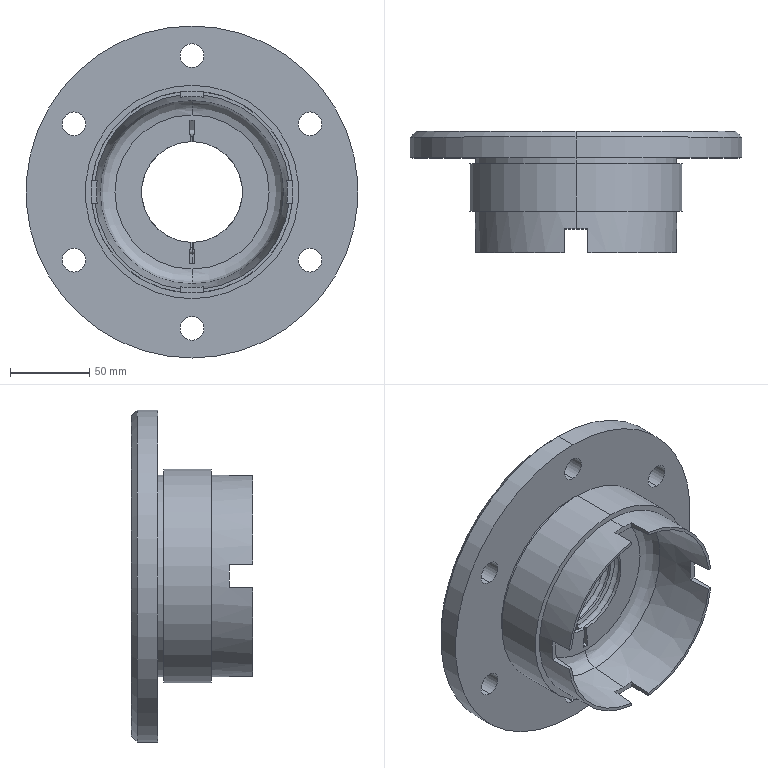Part | SolidWorks | features ICE 3, RevCut 1, Revolution 1, Scale 1 | 1 solid | 83 faces | box 210 x 76.875 x 210 mm | volume 727097 mm3 | cylinder 28 | plane 25 | cone 19 | torus 11 | commonest cylinder face diameters 15 x12 63.75 x8 127.5 x4 135 x2 210 x2